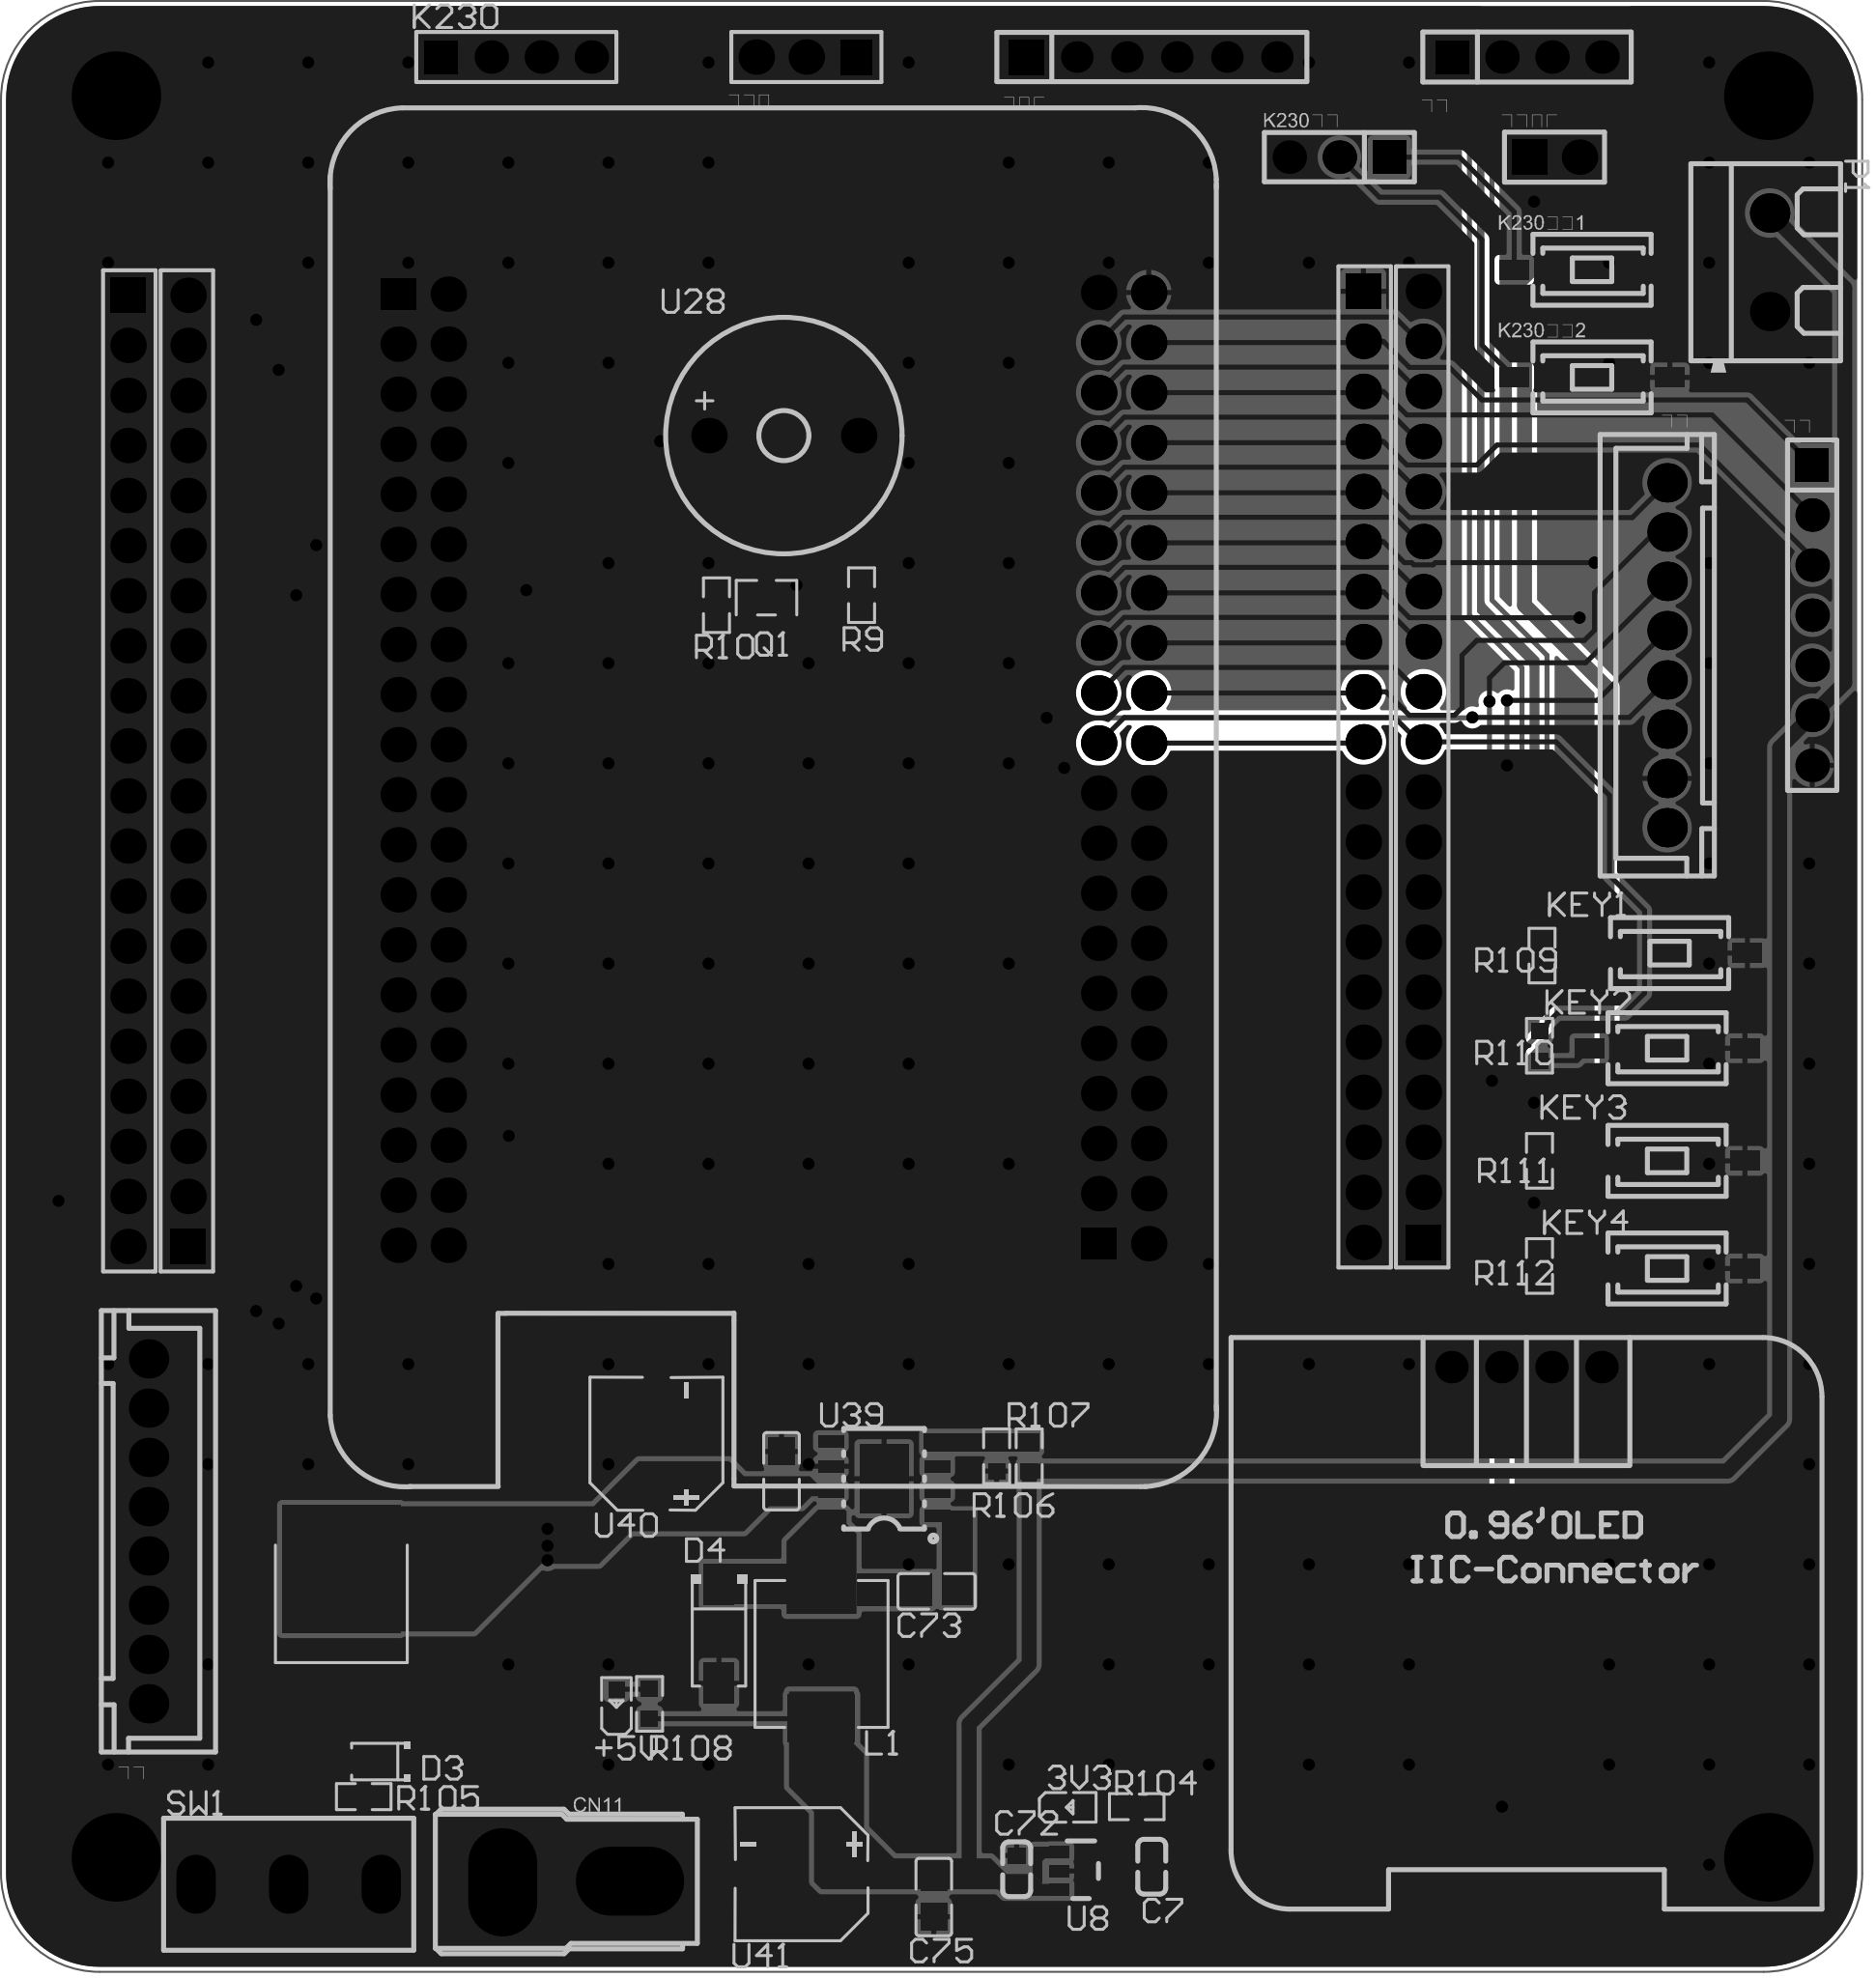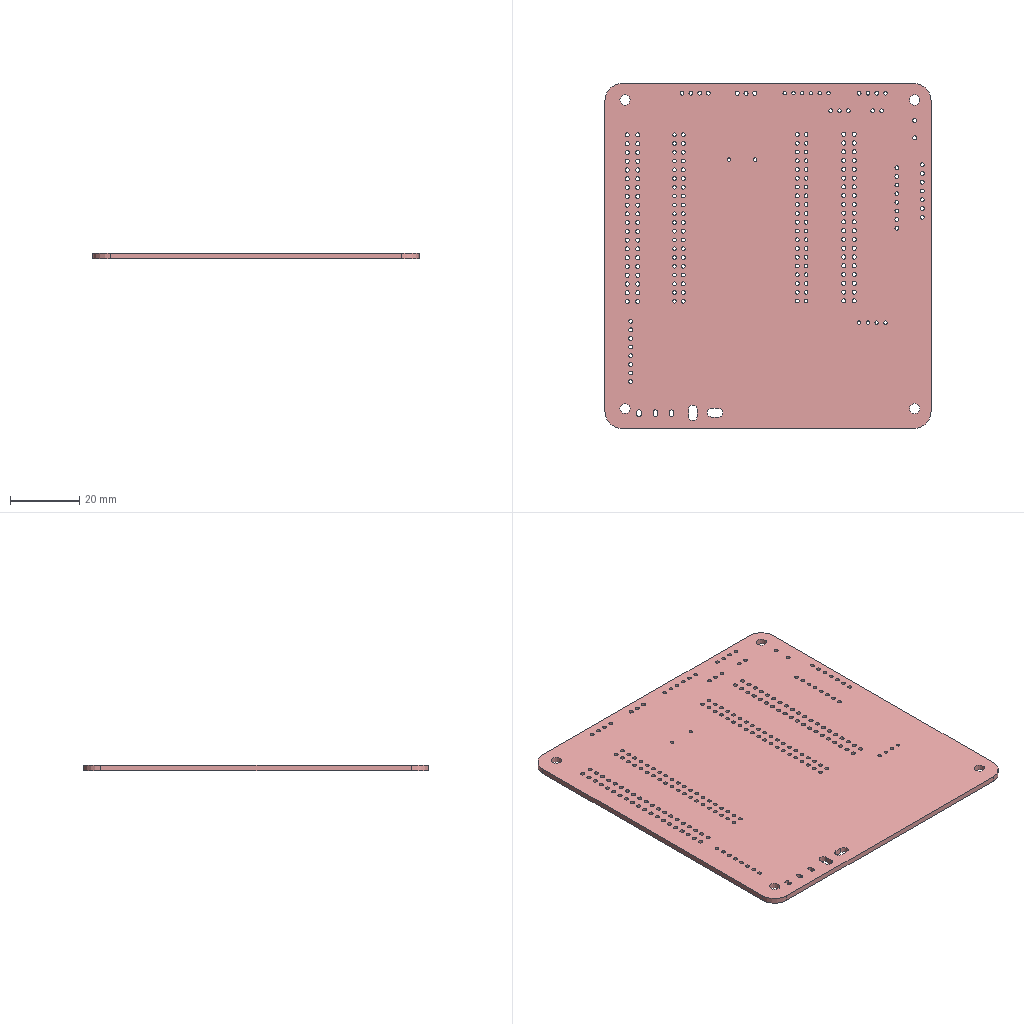Circuit board layout | Altium Designer | box 94.5 x 100 x 1.6 mm
Layer stack:
# Altium Designer layer stack of  (unit mm; dielectric type: 0 none, 1 core, 2 prepreg, 3 surface material)
index,name,kind,layer,copper_thickness_mm,dielectric_type,dielectric_thickness_mm,dielectric_material,dielectric_constant
0,Top Paste Mask Layer,other,,,,,,
1,Top Silkscreen Layer,other,,,,,,
2,Top Solder Mask Layer,dielectric,,,3,0.01,,3.3
3,Top Layer,copper,Top Layer,0.035,,,,
4,Dielectric1,dielectric,,,3,1.51,FR4,4.5
5,Bottom Layer,copper,Bottom Layer,0.035,,,,
6,Bottom Solder Mask Layer,dielectric,,,3,0.01,,3.3
7,Bottom Silkscreen Layer,other,,,,,,
8,Bottom Paste Mask Layer,other,,,,,,
# drill layer pairs: low layer,high layer
drill_pair,Top Layer,Bottom Layer
Part placement:
Designator,Comment,Layer,Footprint,Center-X(mm),Center-Y(mm),Rotation
C7,1uF,TopLayer,C0603,141.351,88.773,90
C72,1uF,TopLayer,C0603,134.493,88.646,270
C73,100nF,TopLayer,C0805,130.429,102.743,180
C74,100nF,TopLayer,C0805,122.555,108.839,270
C75,100nF,TopLayer,C0805,130.286,87.233,90
激光模块,,TopLayer,HDR-TH_2P-P2.54-V-M-1,161.798,175.514,0
CN11,AM-1015B-M,TopLayer,CONN-TH_AM-1015B-M,111.633,88.011,0
D3,BZT52C16,TopLayer,SOD-123_L2.7-W1.6-LS3.7-RD,102.108,94.107,180
D4,SS54,TopLayer,SMA_L4.4-W2.8-LS5.4-R-RD,119.38,100.584,270
H1,,TopLayer,HDR-TH_20P-P2.54-V-M-1,89.383,144.374,270
H2,,TopLayer,HDR-TH_20P-P2.54-V-M-1,92.431,144.374,90
H3,,TopLayer,HDR-TH_20P-P2.54-V-M-1,155.143,144.577,90
H4,,TopLayer,HDR-TH_20P-P2.54-V-M-1,152.095,144.577,270
L1,4.7uH,TopLayer,IND-SMD_L7.3-W6.6,124.587,99.568,90
3V3,,TopLayer,LED_0603,137.135,91.779,0
Q1,S8550,TopLayer,SOT-23-3_L2.9-W1.6-P1.90-LS2.8-BR,121.793,153.162,270
Q2,HY19P03D,TopLayer,TO-252-2_L6.6-W6.1-P4.57-LS9.9-TL-CW,100.203,100.584,90
R9,100Ω,TopLayer,R0603,126.619,153.289,90
R10,100Ω,TopLayer,R0603,119.253,152.781,90
R104,10K,TopLayer,R0603,140.589,91.821,180
R105,10kΩ,TopLayer,R0603,101.346,92.329,180
R106,3.24K,TopLayer,R0603,133.477,109.601,90
R107,10K,TopLayer,R0603,135.128,109.601,270
R108,4.7K,TopLayer,R0603,115.857,97.035,270
U4,,TopLayer,COMM-TH_LCKFB-TMX-MSPM0G3507,122.149,144.475,0
U8,TLV75733PDBVR,TopLayer,SOT-23-5_L2.9-W1.6-P0.95-LS2.8-BL,137.757,88.557,270
K230按键,K230 button,TopLayer,HDR-TH_3P-P2.54-V-M,150.876,175.514,180
P1,KF301-2P terminal block,TopLayer,CONN-TH_XY301V-A-5.0-2P,172.72,170.18,270
R109,100Ω,TopLayer,R0603,161.163,135.001,90
U28,2.6kHz,TopLayer,BUZ-TH_BD12.0-P7.60-D0.6-FD,122.674,161.387,0
R110,100Ω,TopLayer,R0603,161.036,130.429,90
R111,100Ω,TopLayer,R0603,161.036,124.587,90
U39,TPS5430DDAR,TopLayer,ESOP-8_L4.9-W3.9-P1.27-LS6.0-TL-EP,127.762,108.458,180
U40,220uF,TopLayer,CAP-SMD_BD6.3-L6.6-W6.6-LS7.2-FD,116.205,110.236,90
U41,220uF,TopLayer,CAP-SMD_BD6.3-L6.6-W6.6-LS7.2-FD,123.571,88.392,180
SW1,SS-12D10L5,TopLayer,SW-TH_SS-12D10L5,97.536,87.884,180
R112,100Ω,TopLayer,R0603,161.036,119.253,90
+5V,,TopLayer,LED_0603,114.181,96.977,90
驱动板,2.54mm-1*3P straight pin,TopLayer,HDR-TH_3P-P2.54-V-M-1,123.817,180.594,180
测距,PM2.54-1*4,TopLayer,HDR-TH_4P-P2.54-V-F,160.401,180.594,0
灰度,PZ2.54-1*7,TopLayer,HDR-TH_7P-P2.54-V-M,174.879,152.273,270
陀螺仪,2.54-1*6P female,TopLayer,HDR-TH_6P-P2.54-V-F,141.356,180.594,0
KEY3,Tact switch 3*6*2.5,TopLayer,SW-SMD_L6.0-W3.6-LS8.0,167.513,124.587,0
KEY2,Tact switch 3*6*2.5,TopLayer,SW-SMD_L6.0-W3.6-LS8.0,167.513,130.302,0
KEY1,Tact switch 3*6*2.5,TopLayer,SW-SMD_L6.0-W3.6-LS8.0,167.64,135.128,0
K230按键1,Tact switch 3*6*2.5,TopLayer,SW-SMD_L6.0-W3.6-LS8.0,163.703,169.799,0
K230按键2,Tact switch 3*6*2.5,TopLayer,SW-SMD_L6.0-W3.6-LS8.0,163.703,164.338,0
KEY4,Tact switch 3*6*2.5,TopLayer,SW-SMD_L6.0-W3.6-LS8.0,167.513,119.126,0
U5,,TopLayer,0.96OLED_4P,160.375,114.123,0
水平,Horizontal,TopLayer,CONN-TH_8P-P2.50-XH2.54-8P,90.424,105.791,90
竖直,Vertical,TopLayer,CONN-TH_8P-P2.50-XH2.54-8P,167.513,150.241,270
K230,2.54*4 single row,TopLayer,HDR-TH_4P-P2.54-V-M-1,109.093,180.594,0
Pad and via stacks:
# Altium Designer via and pad stacks of  (unit mm). Each distinct definition once, with the count of objects using it.
# via: kind,start_layer,end_layer,hole_mm,diameter_mm,mode(0 simple;1 top-mid-bottom;2 full stack),diameter_per_layer,count,example_net
# pad: kind,layer,hole_mm,hole_type(0 round;1 square;2 slot),plating,top_size,top_shape(1 round;2 rect;3 octagon;9 rounded rect),mid_size,bottom_size,mode,footprint,size_per_layer,count,example
pad,Multi-Layer,3,0,plated,4.501x4.501,1,4.501x4.501,4.501x4.501,0,,,4,1
pad,Multi-Layer,1.1,0,plated,1.8x1.8,1,1.8x1.8,1.8x1.8,0,HDR-TH_2P-P2.54-V-M-1,,1,\u6FC0\u5149\u6A21\u5757.2
pad,Multi-Layer,1.1,0,plated,1.8x1.8,2,1.8x1.8,1.8x1.8,0,HDR-TH_2P-P2.54-V-M-1,,1,\u6FC0\u5149\u6A21\u5757.1
pad,Multi-Layer,2.5,2,plated,3.5x5.5,1,3.5x5.5,3.5x5.5,0,CONN-TH_AM-1015B-M,,2,CN11.1
pad,Multi-Layer,1.2,0,plated,1.8x1.8,1,1.8x1.8,1.8x1.8,0,HDR-TH_20P-P2.54-V-M-1,,76,H1.20
pad,Multi-Layer,1.2,0,plated,1.8x1.8,2,1.8x1.8,1.8x1.8,0,HDR-TH_20P-P2.54-V-M-1,,4,H1.1
pad,Multi-Layer,1.1,0,plated,1.8x1.8,1,1.8x1.8,1.8x1.8,0,COMM-TH_LCKFB-TMX-MSPM0G3507,,78,U4.80
pad,Multi-Layer,1.1,0,plated,1.575x1.8,2,1.575x1.8,1.575x1.8,0,COMM-TH_LCKFB-TMX-MSPM0G3507,,2,U4.41
pad,Multi-Layer,1.1,0,plated,1.7x1.7,2,1.7x1.7,1.7x1.7,0,HDR-TH_3P-P2.54-V-M,,1,K230\u6309\u952E.1
pad,Multi-Layer,1.1,0,plated,1.7x1.7,1,1.7x1.7,1.7x1.7,0,HDR-TH_3P-P2.54-V-M,,2,K230\u6309\u952E.2
pad,Multi-Layer,1.2,0,plated,2x2,1,2x2,2x2,0,CONN-TH_XY301V-A-5.0-2P,,2,P1.1
pad,Multi-Layer,1,0,plated,1.8x1.8,1,1.8x1.8,1.8x1.8,0,BUZ-TH_BD12.0-P7.60-D0.6-FD,,2,U28.2
pad,Multi-Layer,1.3,2,plated,2x3,1,2x3,2x3,0,SW-TH_SS-12D10L5,,3,SW1.1
pad,Multi-Layer,1.2,0,plated,1.8x1.8,1,1.8x1.8,1.8x1.8,0,HDR-TH_3P-P2.54-V-M-1,,2,\u9A71\u52A8\u677F.3
pad,Multi-Layer,1.2,0,plated,1.575x1.8,2,1.575x1.8,1.575x1.8,0,HDR-TH_3P-P2.54-V-M-1,,1,\u9A71\u52A8\u677F.1
pad,Multi-Layer,1.1,0,plated,1.7x1.7,2,1.7x1.7,1.7x1.7,0,HDR-TH_4P-P2.54-V-F,,1,\u6D4B\u8DDD.1
pad,Multi-Layer,1.1,0,plated,1.7x1.7,1,1.7x1.7,1.7x1.7,0,HDR-TH_4P-P2.54-V-F,,3,\u6D4B\u8DDD.2
pad,Multi-Layer,1.1,0,plated,1.7x1.7,2,1.7x1.7,1.7x1.7,0,HDR-TH_7P-P2.54-V-M,,1,\u7070\u5EA6.1
pad,Multi-Layer,1.1,0,plated,1.7x1.7,1,1.7x1.7,1.7x1.7,0,HDR-TH_7P-P2.54-V-M,,6,\u7070\u5EA6.2
pad,Multi-Layer,1.02,0,plated,1.6x1.6,1,1.6x1.6,1.6x1.6,0,HDR-TH_6P-P2.54-V-F,,5,\u9640\u87BA\u4EEA.6
pad,Multi-Layer,1.02,0,plated,1.8x1.8,2,1.8x1.8,1.8x1.8,0,HDR-TH_6P-P2.54-V-F,,1,\u9640\u87BA\u4EEA.1
pad,Multi-Layer,1,0,plated,1.65x1.65,1,1.65x1.65,1.65x1.65,0,0.96OLED_4P,,4,U5.4
pad,Multi-Layer,1.1,0,plated,2x2,1,2x2,2x2,0,CONN-TH_8P-P2.50-XH2.54-8P,,16,\u6C34\u5E73.1
pad,Multi-Layer,1.1,0,plated,1.7x1.7,2,1.7x1.7,1.7x1.7,0,HDR-TH_4P-P2.54-V-M-1,,1,K230.1
pad,Multi-Layer,1.1,0,plated,1.7x1.7,1,1.7x1.7,1.7x1.7,0,HDR-TH_4P-P2.54-V-M-1,,3,K230.2
pad,Top Layer,0,0,plated,0.8x0.9,2,0.8x0.9,0.8x0.9,0,C0603,,4,C7.2
pad,Top Layer,0,0,plated,1.41x1.35,2,1.41x1.35,1.41x1.35,0,C0805,,6,C73.2
pad,Top Layer,0,0,plated,0.91x1.22,2,0.91x1.22,0.91x1.22,0,SOD-123_L2.7-W1.6-LS3.7-RD,,2,D3.2
pad,Top Layer,0,0,plated,2.062x1.539,2,2.062x1.539,2.062x1.539,0,SMA_L4.4-W2.8-LS5.4-R-RD,,2,D4.1
pad,Top Layer,0,0,plated,2.424x3.42,2,2.424x3.42,2.424x3.42,0,IND-SMD_L7.3-W6.6,,2,L1.1
pad,Top Layer,0,0,plated,0.8001x0.8001,2,0.8001x0.8001,0.8001x0.8001,0,LED_0603,,4,3V3.1
pad,Top Layer,0,0,plated,1.07x0.6,2,1.07x0.6,1.07x0.6,0,SOT-23-3_L2.9-W1.6-P1.90-LS2.8-BR,,3,Q1.1
pad,Top Layer,0,0,plated,6.5x6,2,6.5x6,6.5x6,0,TO-252-2_L6.6-W6.1-P4.57-LS9.9-TL-CW,,1,Q2.2
pad,Top Layer,0,0,plated,2.8x1.3,2,2.8x1.3,2.8x1.3,0,TO-252-2_L6.6-W6.1-P4.57-LS9.9-TL-CW,,2,Q2.1
pad,Top Layer,0,0,plated,0.8065x0.864,2,0.8065x0.864,0.8065x0.864,0,R0603,,22,R9.2
pad,Top Layer,0,0,plated,0.6x1,2,0.6x1,0.6x1,0,SOT-23-5_L2.9-W1.6-P0.95-LS2.8-BL,,5,U8.5
pad,Top Layer,0,0,plated,1.3x0.6,2,1.3x0.6,1.3x0.6,0,ESOP-8_L4.9-W3.9-P1.27-LS6.0-TL-EP,,8,U39.1
pad,Top Layer,0,0,plated,2.5x3.5,2,2.5x3.5,2.5x3.5,0,ESOP-8_L4.9-W3.9-P1.27-LS6.0-TL-EP,,1,U39.9
pad,Top Layer,0,0,plated,3.5x1.2,2,3.5x1.2,3.5x1.2,0,CAP-SMD_BD6.3-L6.6-W6.6-LS7.2-FD,,4,U40.2
pad,Top Layer,0,0,plated,1.5x1,2,1.5x1,1.5x1,0,SW-SMD_L6.0-W3.6-LS8.0,,12,KEY3.1
via,Top Layer,Bottom Layer,0.3048,0.61,0,,183,PA15
Copper pours:
name,layer,net,type(0 solid;1 hatched;2 none)
Bottom Layer-GND,Bottom Layer,GND,0
Top Layer-GND,Top Layer,GND,0
Design rules, without the lines most boards share:
# Altium Designer design rules of  (exported by Altium Designer, unit mm)
# columns: name | kind | enabled | priority | scope1 | scope2 | descriptor | typed fields (field=value)
Copper_copperRegion_copperThickness1oz | 0 | disabled | 4 | All | All | Clearance Constraint (Gap=5.984mil) (Disabled)(All),(All) | gap=0.152
Copper_copperRegion_copperThickness1oz_1 | 63 | disabled | 4 | All | All | Board Clearance Constraint (Gap=0mil) (Disabled)(All) |
Copper_copperRegion_Copper_copperRegion | 0 | disabled | 5 | All | All | Clearance Constraint (Gap=5.984mil) (Disabled)(All),(All) | gap=0.152
Copper_copperRegion_Copper_copperRegion_1 | 63 | disabled | 5 | All | All | Board Clearance Constraint (Gap=0mil) (Disabled)(All) |
copperThickness1oz | 0 | enabled | 6 | All | All | Clearance Constraint (Gap=5.984mil) (All),(All) | gap=0.152
copperThickness1oz_1 | 63 | enabled | 6 | All | All | Board Clearance Constraint (Gap=0mil) (All) |
copperRegion_copperThickness1oz | 20 | disabled | 1 | All | All | Polygon Connect Rule(Relief Connect )(Conductor Width=10mil) (Relief Angle=90 Angle) (Entries=4) (Air Gap Width=10mil) (Disabled)(All),(All) | connect_style(0=relief,1=direct,2=none)=0 relief_conductor_width=0.254 relief_entries=4
copperRegion_Copper_copperRegion | 20 | disabled | 2 | All | All | Polygon Connect Rule(Relief Connect )(Conductor Width=10mil) (Relief Angle=90 Angle) (Entries=4) (Air Gap Width=10mil) (Disabled)(All),(All) | connect_style(0=relief,1=direct,2=none)=0 relief_conductor_width=0.254 relief_entries=4
copperRegion | 20 | enabled | 3 | All | All | Polygon Connect Rule(Relief Connect )(Conductor Width=10mil) (Relief Angle=90 Angle) (Entries=4) (Air Gap Width=10mil) (All),(All) | connect_style(0=relief,1=direct,2=none)=0 relief_conductor_width=0.254 relief_entries=4